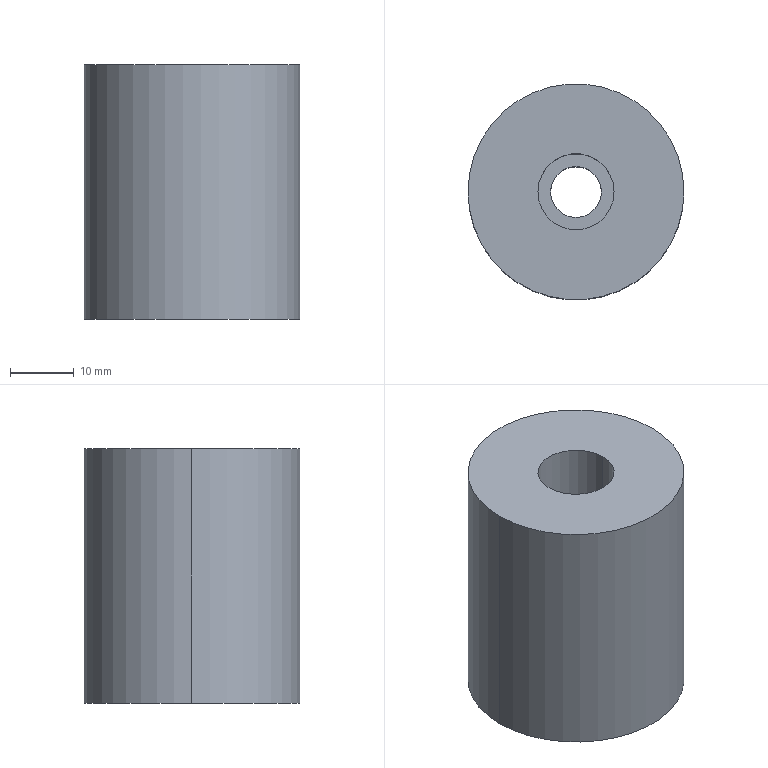Part | 1 solid | 9 faces | box 34 x 34 x 40 mm | volume 33050 mm3 | cylinder 6 | plane 3 | commonest cylinder face diameters 8 x2 12 x2 34 x2
STEP:
#1=CARTESIAN_POINT('',(-6.,0.,20.));
#2=VERTEX_POINT('',#1);
#3=CARTESIAN_POINT('',(6.,0.,20.));
#4=VERTEX_POINT('',#3);
#5=CARTESIAN_POINT('',(0.,0.,20.));
#6=DIRECTION('',(0.,0.,1.));
#7=DIRECTION('',(1.,0.,0.));
#8=AXIS2_PLACEMENT_3D('',#5,#6,#7);
#9=CIRCLE('',#8,6.);
#10=EDGE_CURVE('',#2,#4,#9,.T.);
#11=ORIENTED_EDGE('',*,*,#10,.F.);
#12=CARTESIAN_POINT('',(-6.,0.,40.));
#13=VERTEX_POINT('',#12);
#14=CARTESIAN_POINT('',(-6.,0.,20.));
#15=DIRECTION('',(0.,0.,1.));
#16=VECTOR('',#15,1000.);
#17=LINE('',#14,#16);
#18=EDGE_CURVE('',#2,#13,#17,.T.);
#19=ORIENTED_EDGE('',*,*,#18,.T.);
#20=CARTESIAN_POINT('',(6.,0.,40.));
#21=VERTEX_POINT('',#20);
#22=CARTESIAN_POINT('',(0.,0.,40.));
#23=DIRECTION('',(0.,0.,1.));
#24=DIRECTION('',(1.,0.,0.));
#25=AXIS2_PLACEMENT_3D('',#22,#23,#24);
#26=CIRCLE('',#25,6.);
#27=EDGE_CURVE('',#13,#21,#26,.T.);
#28=ORIENTED_EDGE('',*,*,#27,.T.);
#29=CARTESIAN_POINT('',(6.,0.,20.));
#30=DIRECTION('',(0.,0.,1.));
#31=VECTOR('',#30,1000.);
#32=LINE('',#29,#31);
#33=EDGE_CURVE('',#4,#21,#32,.T.);
#34=ORIENTED_EDGE('',*,*,#33,.F.);
#35=EDGE_LOOP('',(#11,#19,#28,#34));
#36=FACE_OUTER_BOUND('',#35,.T.);
#37=CARTESIAN_POINT('',(0.,0.,20.));
#38=DIRECTION('',(0.,0.,1.));
#39=DIRECTION('',(1.,0.,0.));
#40=AXIS2_PLACEMENT_3D('',#37,#38,#39);
#41=CYLINDRICAL_SURFACE('',#40,6.);
#42=ADVANCED_FACE('',(#36),#41,.F.);
#43=CARTESIAN_POINT('',(4.,0.,20.));
#44=VERTEX_POINT('',#43);
#45=CARTESIAN_POINT('',(-4.,0.,20.));
#46=VERTEX_POINT('',#45);
#47=CARTESIAN_POINT('',(0.,0.,20.));
#48=DIRECTION('',(0.,0.,-1.));
#49=DIRECTION('',(1.,0.,0.));
#50=AXIS2_PLACEMENT_3D('',#47,#48,#49);
#51=CIRCLE('',#50,4.);
#52=EDGE_CURVE('',#44,#46,#51,.T.);
#53=ORIENTED_EDGE('',*,*,#52,.F.);
#54=CARTESIAN_POINT('',(4.,0.,0.));
#55=VERTEX_POINT('',#54);
#56=CARTESIAN_POINT('',(4.,0.,20.));
#57=DIRECTION('',(0.,0.,-1.));
#58=VECTOR('',#57,1000.);
#59=LINE('',#56,#58);
#60=EDGE_CURVE('',#44,#55,#59,.T.);
#61=ORIENTED_EDGE('',*,*,#60,.T.);
#62=CARTESIAN_POINT('',(-4.,0.,0.));
#63=VERTEX_POINT('',#62);
#64=CARTESIAN_POINT('',(0.,0.,0.));
#65=DIRECTION('',(0.,0.,-1.));
#66=DIRECTION('',(-1.,0.,0.));
#67=AXIS2_PLACEMENT_3D('',#64,#65,#66);
#68=CIRCLE('',#67,4.);
#69=EDGE_CURVE('',#55,#63,#68,.T.);
#70=ORIENTED_EDGE('',*,*,#69,.T.);
#71=CARTESIAN_POINT('',(-4.,0.,20.));
#72=DIRECTION('',(0.,0.,-1.));
#73=VECTOR('',#72,1000.);
#74=LINE('',#71,#73);
#75=EDGE_CURVE('',#46,#63,#74,.T.);
#76=ORIENTED_EDGE('',*,*,#75,.F.);
#77=EDGE_LOOP('',(#53,#61,#70,#76));
#78=FACE_OUTER_BOUND('',#77,.T.);
#79=CARTESIAN_POINT('',(0.,0.,20.));
#80=DIRECTION('',(0.,0.,-1.));
#81=DIRECTION('',(-1.,0.,0.));
#82=AXIS2_PLACEMENT_3D('',#79,#80,#81);
#83=CYLINDRICAL_SURFACE('',#82,4.);
#84=ADVANCED_FACE('',(#78),#83,.F.);
#85=CARTESIAN_POINT('',(17.,0.,40.));
#86=VERTEX_POINT('',#85);
#87=CARTESIAN_POINT('',(-17.,0.,40.));
#88=VERTEX_POINT('',#87);
#89=CARTESIAN_POINT('',(0.,0.,40.));
#90=DIRECTION('',(0.,0.,1.));
#91=DIRECTION('',(1.,0.,0.));
#92=AXIS2_PLACEMENT_3D('',#89,#90,#91);
#93=CIRCLE('',#92,17.);
#94=EDGE_CURVE('',#86,#88,#93,.T.);
#95=ORIENTED_EDGE('',*,*,#94,.F.);
#96=CARTESIAN_POINT('',(17.,0.,0.));
#97=VERTEX_POINT('',#96);
#98=CARTESIAN_POINT('',(17.,0.,40.));
#99=DIRECTION('',(0.,0.,-1.));
#100=VECTOR('',#99,1000.);
#101=LINE('',#98,#100);
#102=EDGE_CURVE('',#86,#97,#101,.T.);
#103=ORIENTED_EDGE('',*,*,#102,.T.);
#104=CARTESIAN_POINT('',(-17.,0.,0.));
#105=VERTEX_POINT('',#104);
#106=CARTESIAN_POINT('',(0.,0.,0.));
#107=DIRECTION('',(0.,0.,1.));
#108=DIRECTION('',(1.,0.,0.));
#109=AXIS2_PLACEMENT_3D('',#106,#107,#108);
#110=CIRCLE('',#109,17.);
#111=EDGE_CURVE('',#97,#105,#110,.T.);
#112=ORIENTED_EDGE('',*,*,#111,.T.);
#113=CARTESIAN_POINT('',(-17.,0.,40.));
#114=DIRECTION('',(0.,0.,-1.));
#115=VECTOR('',#114,1000.);
#116=LINE('',#113,#115);
#117=EDGE_CURVE('',#88,#105,#116,.T.);
#118=ORIENTED_EDGE('',*,*,#117,.F.);
#119=EDGE_LOOP('',(#95,#103,#112,#118));
#120=FACE_OUTER_BOUND('',#119,.T.);
#121=CARTESIAN_POINT('',(0.,0.,40.));
#122=DIRECTION('',(0.,0.,-1.));
#123=DIRECTION('',(-1.,0.,0.));
#124=AXIS2_PLACEMENT_3D('',#121,#122,#123);
#125=CYLINDRICAL_SURFACE('',#124,17.);
#126=ADVANCED_FACE('',(#120),#125,.T.);
#127=ORIENTED_EDGE('',*,*,#102,.F.);
#128=CARTESIAN_POINT('',(0.,0.,40.));
#129=DIRECTION('',(0.,0.,1.));
#130=DIRECTION('',(1.,0.,0.));
#131=AXIS2_PLACEMENT_3D('',#128,#129,#130);
#132=CIRCLE('',#131,17.);
#133=EDGE_CURVE('',#88,#86,#132,.T.);
#134=ORIENTED_EDGE('',*,*,#133,.F.);
#135=ORIENTED_EDGE('',*,*,#117,.T.);
#136=CARTESIAN_POINT('',(0.,0.,0.));
#137=DIRECTION('',(0.,0.,1.));
#138=DIRECTION('',(1.,0.,0.));
#139=AXIS2_PLACEMENT_3D('',#136,#137,#138);
#140=CIRCLE('',#139,17.);
#141=EDGE_CURVE('',#105,#97,#140,.T.);
#142=ORIENTED_EDGE('',*,*,#141,.T.);
#143=EDGE_LOOP('',(#127,#134,#135,#142));
#144=FACE_OUTER_BOUND('',#143,.T.);
#145=CARTESIAN_POINT('',(0.,0.,40.));
#146=DIRECTION('',(0.,0.,-1.));
#147=DIRECTION('',(-1.,0.,0.));
#148=AXIS2_PLACEMENT_3D('',#145,#146,#147);
#149=CYLINDRICAL_SURFACE('',#148,17.);
#150=ADVANCED_FACE('',(#144),#149,.T.);
#151=CARTESIAN_POINT('',(0.,0.,40.));
#152=DIRECTION('',(0.,0.,1.));
#153=DIRECTION('',(1.,0.,0.));
#154=AXIS2_PLACEMENT_3D('',#151,#152,#153);
#155=CIRCLE('',#154,6.);
#156=EDGE_CURVE('',#21,#13,#155,.T.);
#157=ORIENTED_EDGE('',*,*,#156,.F.);
#158=ORIENTED_EDGE('',*,*,#27,.F.);
#159=EDGE_LOOP('',(#157,#158));
#160=FACE_BOUND('',#159,.T.);
#161=ORIENTED_EDGE('',*,*,#133,.T.);
#162=ORIENTED_EDGE('',*,*,#94,.T.);
#163=EDGE_LOOP('',(#161,#162));
#164=FACE_OUTER_BOUND('',#163,.T.);
#165=CARTESIAN_POINT('',(0.,0.,40.));
#166=DIRECTION('',(0.,0.,1.));
#167=DIRECTION('',(1.,0.,0.));
#168=AXIS2_PLACEMENT_3D('',#165,#166,#167);
#169=PLANE('',#168);
#170=ADVANCED_FACE('',(#160,#164),#169,.T.);
#171=CARTESIAN_POINT('',(0.,0.,0.));
#172=DIRECTION('',(0.,0.,-1.));
#173=DIRECTION('',(-1.,0.,0.));
#174=AXIS2_PLACEMENT_3D('',#171,#172,#173);
#175=CIRCLE('',#174,4.);
#176=EDGE_CURVE('',#63,#55,#175,.T.);
#177=ORIENTED_EDGE('',*,*,#176,.F.);
#178=ORIENTED_EDGE('',*,*,#69,.F.);
#179=EDGE_LOOP('',(#177,#178));
#180=FACE_BOUND('',#179,.T.);
#181=ORIENTED_EDGE('',*,*,#141,.F.);
#182=ORIENTED_EDGE('',*,*,#111,.F.);
#183=EDGE_LOOP('',(#181,#182));
#184=FACE_OUTER_BOUND('',#183,.T.);
#185=CARTESIAN_POINT('',(0.,0.,0.));
#186=DIRECTION('',(0.,0.,1.));
#187=DIRECTION('',(1.,0.,0.));
#188=AXIS2_PLACEMENT_3D('',#185,#186,#187);
#189=PLANE('',#188);
#190=ADVANCED_FACE('',(#180,#184),#189,.F.);
#191=ORIENTED_EDGE('',*,*,#60,.F.);
#192=CARTESIAN_POINT('',(0.,0.,20.));
#193=DIRECTION('',(0.,0.,-1.));
#194=DIRECTION('',(1.,0.,0.));
#195=AXIS2_PLACEMENT_3D('',#192,#193,#194);
#196=CIRCLE('',#195,4.);
#197=EDGE_CURVE('',#46,#44,#196,.T.);
#198=ORIENTED_EDGE('',*,*,#197,.F.);
#199=ORIENTED_EDGE('',*,*,#75,.T.);
#200=ORIENTED_EDGE('',*,*,#176,.T.);
#201=EDGE_LOOP('',(#191,#198,#199,#200));
#202=FACE_OUTER_BOUND('',#201,.T.);
#203=CARTESIAN_POINT('',(0.,0.,20.));
#204=DIRECTION('',(0.,0.,-1.));
#205=DIRECTION('',(-1.,0.,0.));
#206=AXIS2_PLACEMENT_3D('',#203,#204,#205);
#207=CYLINDRICAL_SURFACE('',#206,4.);
#208=ADVANCED_FACE('',(#202),#207,.F.);
#209=CARTESIAN_POINT('',(0.,0.,20.));
#210=DIRECTION('',(0.,0.,1.));
#211=DIRECTION('',(1.,0.,0.));
#212=AXIS2_PLACEMENT_3D('',#209,#210,#211);
#213=CIRCLE('',#212,6.);
#214=EDGE_CURVE('',#4,#2,#213,.T.);
#215=ORIENTED_EDGE('',*,*,#214,.T.);
#216=ORIENTED_EDGE('',*,*,#10,.T.);
#217=EDGE_LOOP('',(#215,#216));
#218=FACE_OUTER_BOUND('',#217,.T.);
#219=ORIENTED_EDGE('',*,*,#197,.T.);
#220=ORIENTED_EDGE('',*,*,#52,.T.);
#221=EDGE_LOOP('',(#219,#220));
#222=FACE_BOUND('',#221,.T.);
#223=CARTESIAN_POINT('',(0.,0.,20.));
#224=DIRECTION('',(0.,0.,1.));
#225=DIRECTION('',(1.,0.,0.));
#226=AXIS2_PLACEMENT_3D('',#223,#224,#225);
#227=PLANE('',#226);
#228=ADVANCED_FACE('',(#218,#222),#227,.T.);
#229=ORIENTED_EDGE('',*,*,#18,.F.);
#230=ORIENTED_EDGE('',*,*,#214,.F.);
#231=ORIENTED_EDGE('',*,*,#33,.T.);
#232=ORIENTED_EDGE('',*,*,#156,.T.);
#233=EDGE_LOOP('',(#229,#230,#231,#232));
#234=FACE_OUTER_BOUND('',#233,.T.);
#235=CARTESIAN_POINT('',(0.,0.,20.));
#236=DIRECTION('',(0.,0.,1.));
#237=DIRECTION('',(1.,0.,0.));
#238=AXIS2_PLACEMENT_3D('',#235,#236,#237);
#239=CYLINDRICAL_SURFACE('',#238,6.);
#240=ADVANCED_FACE('',(#234),#239,.F.);
#241=CLOSED_SHELL('',(#42,#84,#126,#150,#170,#190,#208,#228,#240));
#242=MANIFOLD_SOLID_BREP('',#241);
#243=CARTESIAN_POINT('',(0.,0.,0.));
#244=DIRECTION('',(0.,0.,1.));
#245=DIRECTION('',(1.,0.,0.));
#246=AXIS2_PLACEMENT_3D('',#243,#244,#245);
#247=(LENGTH_UNIT()NAMED_UNIT(*)SI_UNIT(.MILLI.,.METRE.));
#248=UNCERTAINTY_MEASURE_WITH_UNIT(LENGTH_MEASURE(0.00001),#247,'','');
#249=(NAMED_UNIT(*)PLANE_ANGLE_UNIT()SI_UNIT($,.RADIAN.));
#250=(NAMED_UNIT(*)SI_UNIT($,.STERADIAN.)SOLID_ANGLE_UNIT());
#251=(GEOMETRIC_REPRESENTATION_CONTEXT(3)GLOBAL_UNCERTAINTY_ASSIGNED_CONTEXT((#248))GLOBAL_UNIT_ASSIGNED_CONTEXT((#247,#249,#250))REPRESENTATION_CONTEXT('',''));
#252=ADVANCED_BREP_SHAPE_REPRESENTATION('',(#242,#246),#251);